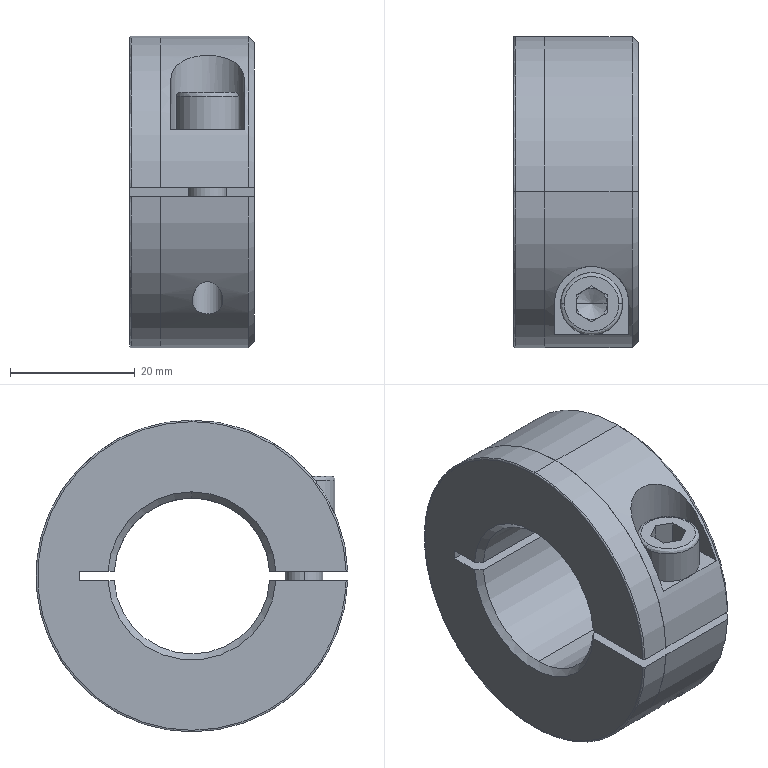Part | SolidWorks | features BaseBody 2 | 2 solids | 70 faces | box 20 x 50.04 x 50.051 mm | volume 28246 mm3 | plane 26 | cylinder 18 | cone 17 | spline 9 | commonest cylinder face diameters 25.02 x3 50 x3 50.051 x3 4.917 x2 6 x2 7 x2